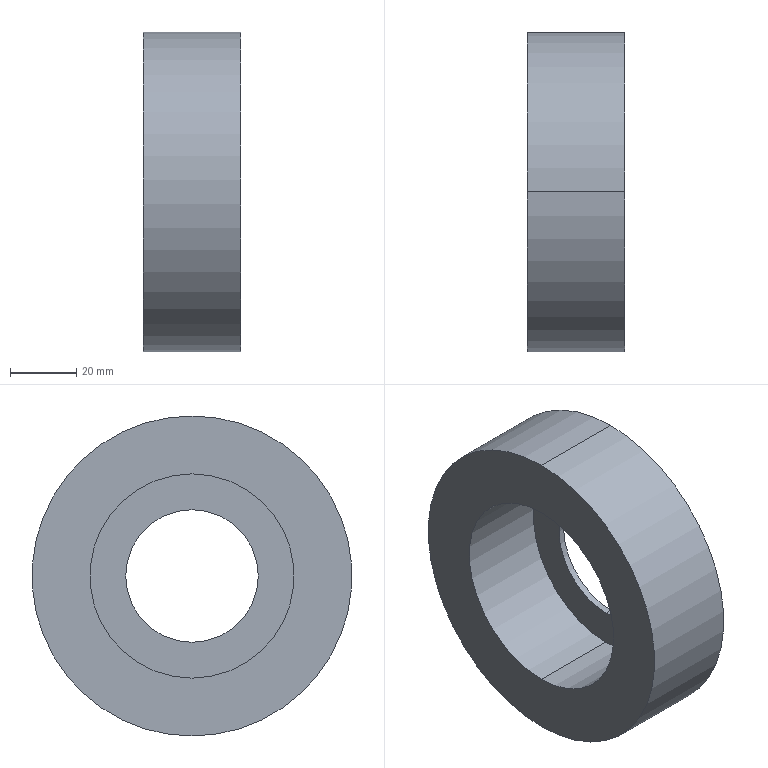Part | STEP file | Market stator | 1 solid | 9 faces | box 29.5 x 96.5 x 96.5 mm | volume 131288 mm3 | cylinder 6 | plane 3 | commonest cylinder face diameters 40 x2 61.6 x2 96.5 x2
STEP:
#1=CARTESIAN_POINT('',(0.,0.,0.));
#2=DIRECTION('',(0.,0.,1.));
#3=DIRECTION('',(1.,0.,0.));
#4=AXIS2_PLACEMENT_3D('',#1,#2,#3);
#5=CARTESIAN_POINT('',(-2.,0.,-20.));
#6=VERTEX_POINT('',#5);
#7=CARTESIAN_POINT('',(0.,0.,-20.));
#8=VERTEX_POINT('',#7);
#9=CARTESIAN_POINT('',(0.,0.,-20.));
#10=DIRECTION('',(1.,0.,0.));
#11=VECTOR('',#10,1.);
#12=LINE('',#9,#11);
#13=CARTESIAN_POINT('',(0.,0.,0.));
#14=DIRECTION('',(1.,0.,0.));
#15=DIRECTION('',(0.,0.,-1.));
#16=AXIS2_PLACEMENT_3D('',#13,#14,#15);
#17=CYLINDRICAL_SURFACE('',#16,20.);
#18=CARTESIAN_POINT('',(6.283,0.));
#19=DIRECTION('',(0.,1.));
#20=VECTOR('',#19,1.);
#21=LINE('',#18,#20);
#22=(GEOMETRIC_REPRESENTATION_CONTEXT(2)PARAMETRIC_REPRESENTATION_CONTEXT()REPRESENTATION_CONTEXT('',''));
#23=DEFINITIONAL_REPRESENTATION('',(#21),#22);
#24=PCURVE('',#17,#23);
#25=CARTESIAN_POINT('',(0.,0.,0.));
#26=DIRECTION('',(1.,0.,0.));
#27=DIRECTION('',(0.,0.,-1.));
#28=AXIS2_PLACEMENT_3D('',#25,#26,#27);
#29=CYLINDRICAL_SURFACE('',#28,20.);
#30=CARTESIAN_POINT('',(0.,0.));
#31=DIRECTION('',(0.,1.));
#32=VECTOR('',#31,1.);
#33=LINE('',#30,#32);
#34=(GEOMETRIC_REPRESENTATION_CONTEXT(2)PARAMETRIC_REPRESENTATION_CONTEXT()REPRESENTATION_CONTEXT('',''));
#35=DEFINITIONAL_REPRESENTATION('',(#33),#34);
#36=PCURVE('',#29,#35);
#37=SURFACE_CURVE('',#12,(#24,#36),.PCURVE_S1.);
#38=EDGE_CURVE('',#6,#8,#37,.T.);
#39=ORIENTED_EDGE('',*,*,#38,.T.);
#40=CARTESIAN_POINT('',(0.,0.,20.));
#41=VERTEX_POINT('',#40);
#42=CARTESIAN_POINT('',(0.,0.,0.));
#43=DIRECTION('',(-1.,0.,0.));
#44=DIRECTION('',(0.,0.,-1.));
#45=AXIS2_PLACEMENT_3D('',#42,#43,#44);
#46=CIRCLE('',#45,20.);
#47=CARTESIAN_POINT('',(6.283,0.));
#48=DIRECTION('',(-1.,0.));
#49=VECTOR('',#48,1.);
#50=LINE('',#47,#49);
#51=(GEOMETRIC_REPRESENTATION_CONTEXT(2)PARAMETRIC_REPRESENTATION_CONTEXT()REPRESENTATION_CONTEXT('',''));
#52=DEFINITIONAL_REPRESENTATION('',(#50),#51);
#53=PCURVE('',#17,#52);
#54=CARTESIAN_POINT('',(0.,20.,0.));
#55=DIRECTION('',(1.,0.,0.));
#56=DIRECTION('',(0.,0.,-1.));
#57=AXIS2_PLACEMENT_3D('',#54,#55,#56);
#58=PLANE('',#57);
#59=CARTESIAN_POINT('',(20.,-20.));
#60=CARTESIAN_POINT('',(20.,-54.641));
#61=CARTESIAN_POINT('',(-10.,-37.321));
#62=CARTESIAN_POINT('',(-40.,-20.));
#63=CARTESIAN_POINT('',(-10.,-2.679));
#64=CARTESIAN_POINT('',(20.,14.641));
#65=CARTESIAN_POINT('',(20.,-20.));
#66=(BOUNDED_CURVE()B_SPLINE_CURVE(2,(#59,#60,#61,#62,#63,#64,#65),.UNSPECIFIED.,.T.,.F.)B_SPLINE_CURVE_WITH_KNOTS((1,2,2,2,2,1),(-2.094,0.,2.094,4.189,6.283,8.378),.UNSPECIFIED.)CURVE()GEOMETRIC_REPRESENTATION_ITEM()RATIONAL_B_SPLINE_CURVE((1.,0.5,1.,0.5,1.,0.5,1.))REPRESENTATION_ITEM(''));
#67=(GEOMETRIC_REPRESENTATION_CONTEXT(2)PARAMETRIC_REPRESENTATION_CONTEXT()REPRESENTATION_CONTEXT('',''));
#68=DEFINITIONAL_REPRESENTATION('',(#66),#67);
#69=PCURVE('',#58,#68);
#70=SURFACE_CURVE('',#46,(#53,#69),.PCURVE_S1.);
#71=EDGE_CURVE('',#8,#41,#70,.T.);
#72=ORIENTED_EDGE('',*,*,#71,.T.);
#73=CARTESIAN_POINT('',(-2.,0.,20.));
#74=VERTEX_POINT('',#73);
#75=CARTESIAN_POINT('',(0.,0.,20.));
#76=DIRECTION('',(1.,0.,0.));
#77=VECTOR('',#76,1.);
#78=LINE('',#75,#77);
#79=CARTESIAN_POINT('',(3.142,0.));
#80=DIRECTION('',(0.,1.));
#81=VECTOR('',#80,1.);
#82=LINE('',#79,#81);
#83=(GEOMETRIC_REPRESENTATION_CONTEXT(2)PARAMETRIC_REPRESENTATION_CONTEXT()REPRESENTATION_CONTEXT('',''));
#84=DEFINITIONAL_REPRESENTATION('',(#82),#83);
#85=PCURVE('',#17,#84);
#86=CARTESIAN_POINT('',(3.142,0.));
#87=DIRECTION('',(0.,1.));
#88=VECTOR('',#87,1.);
#89=LINE('',#86,#88);
#90=(GEOMETRIC_REPRESENTATION_CONTEXT(2)PARAMETRIC_REPRESENTATION_CONTEXT()REPRESENTATION_CONTEXT('',''));
#91=DEFINITIONAL_REPRESENTATION('',(#89),#90);
#92=PCURVE('',#29,#91);
#93=SURFACE_CURVE('',#78,(#85,#92),.PCURVE_S1.);
#94=EDGE_CURVE('',#74,#41,#93,.T.);
#95=ORIENTED_EDGE('',*,*,#94,.F.);
#96=CARTESIAN_POINT('',(-2.,0.,0.));
#97=DIRECTION('',(1.,0.,0.));
#98=DIRECTION('',(0.,0.,-1.));
#99=AXIS2_PLACEMENT_3D('',#96,#97,#98);
#100=CIRCLE('',#99,20.);
#101=CARTESIAN_POINT('',(0.,-2.));
#102=DIRECTION('',(1.,0.));
#103=VECTOR('',#102,1.);
#104=LINE('',#101,#103);
#105=(GEOMETRIC_REPRESENTATION_CONTEXT(2)PARAMETRIC_REPRESENTATION_CONTEXT()REPRESENTATION_CONTEXT('',''));
#106=DEFINITIONAL_REPRESENTATION('',(#104),#105);
#107=PCURVE('',#17,#106);
#108=CARTESIAN_POINT('',(-2.,30.8,0.));
#109=DIRECTION('',(-1.,0.,0.));
#110=DIRECTION('',(0.,0.,1.));
#111=AXIS2_PLACEMENT_3D('',#108,#109,#110);
#112=PLANE('',#111);
#113=CARTESIAN_POINT('',(-20.,-30.8));
#114=CARTESIAN_POINT('',(-20.,3.841));
#115=CARTESIAN_POINT('',(10.,-13.479));
#116=CARTESIAN_POINT('',(40.,-30.8));
#117=CARTESIAN_POINT('',(10.,-48.121));
#118=CARTESIAN_POINT('',(-20.,-65.441));
#119=CARTESIAN_POINT('',(-20.,-30.8));
#120=(BOUNDED_CURVE()B_SPLINE_CURVE(2,(#113,#114,#115,#116,#117,#118,#119),.UNSPECIFIED.,.T.,.F.)B_SPLINE_CURVE_WITH_KNOTS((1,2,2,2,2,1),(-2.094,0.,2.094,4.189,6.283,8.378),.UNSPECIFIED.)CURVE()GEOMETRIC_REPRESENTATION_ITEM()RATIONAL_B_SPLINE_CURVE((1.,0.5,1.,0.5,1.,0.5,1.))REPRESENTATION_ITEM(''));
#121=(GEOMETRIC_REPRESENTATION_CONTEXT(2)PARAMETRIC_REPRESENTATION_CONTEXT()REPRESENTATION_CONTEXT('',''));
#122=DEFINITIONAL_REPRESENTATION('',(#120),#121);
#123=PCURVE('',#112,#122);
#124=SURFACE_CURVE('',#100,(#107,#123),.PCURVE_S1.);
#125=EDGE_CURVE('',#74,#6,#124,.T.);
#126=ORIENTED_EDGE('',*,*,#125,.T.);
#127=EDGE_LOOP('',(#39,#72,#95,#126));
#128=FACE_BOUND('',#127,.F.);
#129=ADVANCED_FACE('',(#128),#17,.F.);
#130=CARTESIAN_POINT('',(-29.5,0.,-48.25));
#131=VERTEX_POINT('',#130);
#132=CARTESIAN_POINT('',(-29.5,0.,48.25));
#133=VERTEX_POINT('',#132);
#134=CARTESIAN_POINT('',(-29.5,0.,0.));
#135=DIRECTION('',(1.,0.,0.));
#136=DIRECTION('',(0.,0.,-1.));
#137=AXIS2_PLACEMENT_3D('',#134,#135,#136);
#138=CIRCLE('',#137,48.25);
#139=CARTESIAN_POINT('',(0.,0.,0.));
#140=DIRECTION('',(1.,0.,0.));
#141=DIRECTION('',(0.,0.,-1.));
#142=AXIS2_PLACEMENT_3D('',#139,#140,#141);
#143=CYLINDRICAL_SURFACE('',#142,48.25);
#144=CARTESIAN_POINT('',(0.,-29.5));
#145=DIRECTION('',(1.,0.));
#146=VECTOR('',#145,1.);
#147=LINE('',#144,#146);
#148=(GEOMETRIC_REPRESENTATION_CONTEXT(2)PARAMETRIC_REPRESENTATION_CONTEXT()REPRESENTATION_CONTEXT('',''));
#149=DEFINITIONAL_REPRESENTATION('',(#147),#148);
#150=PCURVE('',#143,#149);
#151=CARTESIAN_POINT('',(-29.5,48.25,0.));
#152=DIRECTION('',(-1.,0.,0.));
#153=DIRECTION('',(0.,0.,1.));
#154=AXIS2_PLACEMENT_3D('',#151,#152,#153);
#155=PLANE('',#154);
#156=CARTESIAN_POINT('',(-48.25,-48.25));
#157=CARTESIAN_POINT('',(-48.25,35.321));
#158=CARTESIAN_POINT('',(24.125,-6.464));
#159=CARTESIAN_POINT('',(96.5,-48.25));
#160=CARTESIAN_POINT('',(24.125,-90.036));
#161=CARTESIAN_POINT('',(-48.25,-131.821));
#162=CARTESIAN_POINT('',(-48.25,-48.25));
#163=(BOUNDED_CURVE()B_SPLINE_CURVE(2,(#156,#157,#158,#159,#160,#161,#162),.UNSPECIFIED.,.T.,.F.)B_SPLINE_CURVE_WITH_KNOTS((1,2,2,2,2,1),(-2.094,0.,2.094,4.189,6.283,8.378),.UNSPECIFIED.)CURVE()GEOMETRIC_REPRESENTATION_ITEM()RATIONAL_B_SPLINE_CURVE((1.,0.5,1.,0.5,1.,0.5,1.))REPRESENTATION_ITEM(''));
#164=(GEOMETRIC_REPRESENTATION_CONTEXT(2)PARAMETRIC_REPRESENTATION_CONTEXT()REPRESENTATION_CONTEXT('',''));
#165=DEFINITIONAL_REPRESENTATION('',(#163),#164);
#166=PCURVE('',#155,#165);
#167=SURFACE_CURVE('',#138,(#150,#166),.PCURVE_S1.);
#168=EDGE_CURVE('',#131,#133,#167,.T.);
#169=ORIENTED_EDGE('',*,*,#168,.T.);
#170=CARTESIAN_POINT('',(0.,0.,48.25));
#171=VERTEX_POINT('',#170);
#172=CARTESIAN_POINT('',(0.,0.,48.25));
#173=DIRECTION('',(1.,0.,0.));
#174=VECTOR('',#173,1.);
#175=LINE('',#172,#174);
#176=CARTESIAN_POINT('',(3.142,0.));
#177=DIRECTION('',(0.,1.));
#178=VECTOR('',#177,1.);
#179=LINE('',#176,#178);
#180=(GEOMETRIC_REPRESENTATION_CONTEXT(2)PARAMETRIC_REPRESENTATION_CONTEXT()REPRESENTATION_CONTEXT('',''));
#181=DEFINITIONAL_REPRESENTATION('',(#179),#180);
#182=PCURVE('',#143,#181);
#183=CARTESIAN_POINT('',(0.,0.,0.));
#184=DIRECTION('',(1.,0.,0.));
#185=DIRECTION('',(0.,0.,-1.));
#186=AXIS2_PLACEMENT_3D('',#183,#184,#185);
#187=CYLINDRICAL_SURFACE('',#186,48.25);
#188=CARTESIAN_POINT('',(3.142,0.));
#189=DIRECTION('',(0.,1.));
#190=VECTOR('',#189,1.);
#191=LINE('',#188,#190);
#192=(GEOMETRIC_REPRESENTATION_CONTEXT(2)PARAMETRIC_REPRESENTATION_CONTEXT()REPRESENTATION_CONTEXT('',''));
#193=DEFINITIONAL_REPRESENTATION('',(#191),#192);
#194=PCURVE('',#187,#193);
#195=SURFACE_CURVE('',#175,(#182,#194),.PCURVE_S1.);
#196=EDGE_CURVE('',#133,#171,#195,.T.);
#197=ORIENTED_EDGE('',*,*,#196,.T.);
#198=CARTESIAN_POINT('',(0.,0.,-48.25));
#199=VERTEX_POINT('',#198);
#200=CARTESIAN_POINT('',(0.,0.,0.));
#201=DIRECTION('',(1.,0.,0.));
#202=DIRECTION('',(0.,0.,-1.));
#203=AXIS2_PLACEMENT_3D('',#200,#201,#202);
#204=CIRCLE('',#203,48.25);
#205=CARTESIAN_POINT('',(0.,0.));
#206=DIRECTION('',(1.,0.));
#207=VECTOR('',#206,1.);
#208=LINE('',#205,#207);
#209=(GEOMETRIC_REPRESENTATION_CONTEXT(2)PARAMETRIC_REPRESENTATION_CONTEXT()REPRESENTATION_CONTEXT('',''));
#210=DEFINITIONAL_REPRESENTATION('',(#208),#209);
#211=PCURVE('',#143,#210);
#212=CARTESIAN_POINT('',(0.,-20.));
#213=DIRECTION('',(1.,0.));
#214=AXIS2_PLACEMENT_2D('',#212,#213);
#215=CIRCLE('',#214,48.25);
#216=(GEOMETRIC_REPRESENTATION_CONTEXT(2)PARAMETRIC_REPRESENTATION_CONTEXT()REPRESENTATION_CONTEXT('',''));
#217=DEFINITIONAL_REPRESENTATION('',(#215),#216);
#218=PCURVE('',#58,#217);
#219=SURFACE_CURVE('',#204,(#211,#218),.PCURVE_S1.);
#220=EDGE_CURVE('',#199,#171,#219,.T.);
#221=ORIENTED_EDGE('',*,*,#220,.F.);
#222=CARTESIAN_POINT('',(0.,0.,-48.25));
#223=DIRECTION('',(1.,0.,0.));
#224=VECTOR('',#223,1.);
#225=LINE('',#222,#224);
#226=CARTESIAN_POINT('',(0.,0.));
#227=DIRECTION('',(0.,1.));
#228=VECTOR('',#227,1.);
#229=LINE('',#226,#228);
#230=(GEOMETRIC_REPRESENTATION_CONTEXT(2)PARAMETRIC_REPRESENTATION_CONTEXT()REPRESENTATION_CONTEXT('',''));
#231=DEFINITIONAL_REPRESENTATION('',(#229),#230);
#232=PCURVE('',#143,#231);
#233=CARTESIAN_POINT('',(6.283,0.));
#234=DIRECTION('',(0.,1.));
#235=VECTOR('',#234,1.);
#236=LINE('',#233,#235);
#237=(GEOMETRIC_REPRESENTATION_CONTEXT(2)PARAMETRIC_REPRESENTATION_CONTEXT()REPRESENTATION_CONTEXT('',''));
#238=DEFINITIONAL_REPRESENTATION('',(#236),#237);
#239=PCURVE('',#187,#238);
#240=SURFACE_CURVE('',#225,(#232,#239),.PCURVE_S1.);
#241=EDGE_CURVE('',#131,#199,#240,.T.);
#242=ORIENTED_EDGE('',*,*,#241,.F.);
#243=EDGE_LOOP('',(#169,#197,#221,#242));
#244=FACE_BOUND('',#243,.T.);
#245=ADVANCED_FACE('',(#244),#143,.T.);
#246=CARTESIAN_POINT('',(-29.5,0.,-30.8));
#247=VERTEX_POINT('',#246);
#248=CARTESIAN_POINT('',(-2.,0.,-30.8));
#249=VERTEX_POINT('',#248);
#250=CARTESIAN_POINT('',(0.,0.,-30.8));
#251=DIRECTION('',(1.,0.,0.));
#252=VECTOR('',#251,1.);
#253=LINE('',#250,#252);
#254=CARTESIAN_POINT('',(0.,0.,0.));
#255=DIRECTION('',(1.,0.,0.));
#256=DIRECTION('',(0.,0.,-1.));
#257=AXIS2_PLACEMENT_3D('',#254,#255,#256);
#258=CYLINDRICAL_SURFACE('',#257,30.8);
#259=CARTESIAN_POINT('',(6.283,0.));
#260=DIRECTION('',(0.,1.));
#261=VECTOR('',#260,1.);
#262=LINE('',#259,#261);
#263=(GEOMETRIC_REPRESENTATION_CONTEXT(2)PARAMETRIC_REPRESENTATION_CONTEXT()REPRESENTATION_CONTEXT('',''));
#264=DEFINITIONAL_REPRESENTATION('',(#262),#263);
#265=PCURVE('',#258,#264);
#266=CARTESIAN_POINT('',(0.,0.,0.));
#267=DIRECTION('',(1.,0.,0.));
#268=DIRECTION('',(0.,0.,-1.));
#269=AXIS2_PLACEMENT_3D('',#266,#267,#268);
#270=CYLINDRICAL_SURFACE('',#269,30.8);
#271=CARTESIAN_POINT('',(0.,0.));
#272=DIRECTION('',(0.,1.));
#273=VECTOR('',#272,1.);
#274=LINE('',#271,#273);
#275=(GEOMETRIC_REPRESENTATION_CONTEXT(2)PARAMETRIC_REPRESENTATION_CONTEXT()REPRESENTATION_CONTEXT('',''));
#276=DEFINITIONAL_REPRESENTATION('',(#274),#275);
#277=PCURVE('',#270,#276);
#278=SURFACE_CURVE('',#253,(#265,#277),.PCURVE_S1.);
#279=EDGE_CURVE('',#247,#249,#278,.T.);
#280=ORIENTED_EDGE('',*,*,#279,.T.);
#281=CARTESIAN_POINT('',(-2.,0.,30.8));
#282=VERTEX_POINT('',#281);
#283=CARTESIAN_POINT('',(-2.,0.,0.));
#284=DIRECTION('',(-1.,0.,0.));
#285=DIRECTION('',(0.,0.,-1.));
#286=AXIS2_PLACEMENT_3D('',#283,#284,#285);
#287=CIRCLE('',#286,30.8);
#288=CARTESIAN_POINT('',(6.283,-2.));
#289=DIRECTION('',(-1.,0.));
#290=VECTOR('',#289,1.);
#291=LINE('',#288,#290);
#292=(GEOMETRIC_REPRESENTATION_CONTEXT(2)PARAMETRIC_REPRESENTATION_CONTEXT()REPRESENTATION_CONTEXT('',''));
#293=DEFINITIONAL_REPRESENTATION('',(#291),#292);
#294=PCURVE('',#258,#293);
#295=CARTESIAN_POINT('',(0.,-30.8));
#296=DIRECTION('',(-1.,0.));
#297=AXIS2_PLACEMENT_2D('',#295,#296);
#298=CIRCLE('',#297,30.8);
#299=(GEOMETRIC_REPRESENTATION_CONTEXT(2)PARAMETRIC_REPRESENTATION_CONTEXT()REPRESENTATION_CONTEXT('',''));
#300=DEFINITIONAL_REPRESENTATION('',(#298),#299);
#301=PCURVE('',#112,#300);
#302=SURFACE_CURVE('',#287,(#294,#301),.PCURVE_S1.);
#303=EDGE_CURVE('',#249,#282,#302,.T.);
#304=ORIENTED_EDGE('',*,*,#303,.T.);
#305=CARTESIAN_POINT('',(-29.5,0.,30.8));
#306=VERTEX_POINT('',#305);
#307=CARTESIAN_POINT('',(0.,0.,30.8));
#308=DIRECTION('',(1.,0.,0.));
#309=VECTOR('',#308,1.);
#310=LINE('',#307,#309);
#311=CARTESIAN_POINT('',(3.142,0.));
#312=DIRECTION('',(0.,1.));
#313=VECTOR('',#312,1.);
#314=LINE('',#311,#313);
#315=(GEOMETRIC_REPRESENTATION_CONTEXT(2)PARAMETRIC_REPRESENTATION_CONTEXT()REPRESENTATION_CONTEXT('',''));
#316=DEFINITIONAL_REPRESENTATION('',(#314),#315);
#317=PCURVE('',#258,#316);
#318=CARTESIAN_POINT('',(3.142,0.));
#319=DIRECTION('',(0.,1.));
#320=VECTOR('',#319,1.);
#321=LINE('',#318,#320);
#322=(GEOMETRIC_REPRESENTATION_CONTEXT(2)PARAMETRIC_REPRESENTATION_CONTEXT()REPRESENTATION_CONTEXT('',''));
#323=DEFINITIONAL_REPRESENTATION('',(#321),#322);
#324=PCURVE('',#270,#323);
#325=SURFACE_CURVE('',#310,(#317,#324),.PCURVE_S1.);
#326=EDGE_CURVE('',#306,#282,#325,.T.);
#327=ORIENTED_EDGE('',*,*,#326,.F.);
#328=CARTESIAN_POINT('',(-29.5,0.,0.));
#329=DIRECTION('',(1.,0.,0.));
#330=DIRECTION('',(0.,0.,-1.));
#331=AXIS2_PLACEMENT_3D('',#328,#329,#330);
#332=CIRCLE('',#331,30.8);
#333=CARTESIAN_POINT('',(0.,-29.5));
#334=DIRECTION('',(1.,0.));
#335=VECTOR('',#334,1.);
#336=LINE('',#333,#335);
#337=(GEOMETRIC_REPRESENTATION_CONTEXT(2)PARAMETRIC_REPRESENTATION_CONTEXT()REPRESENTATION_CONTEXT('',''));
#338=DEFINITIONAL_REPRESENTATION('',(#336),#337);
#339=PCURVE('',#258,#338);
#340=CARTESIAN_POINT('',(-30.8,-48.25));
#341=CARTESIAN_POINT('',(-30.8,5.097));
#342=CARTESIAN_POINT('',(15.4,-21.576));
#343=CARTESIAN_POINT('',(61.6,-48.25));
#344=CARTESIAN_POINT('',(15.4,-74.924));
#345=CARTESIAN_POINT('',(-30.8,-101.597));
#346=CARTESIAN_POINT('',(-30.8,-48.25));
#347=(BOUNDED_CURVE()B_SPLINE_CURVE(2,(#340,#341,#342,#343,#344,#345,#346),.UNSPECIFIED.,.T.,.F.)B_SPLINE_CURVE_WITH_KNOTS((1,2,2,2,2,1),(-2.094,0.,2.094,4.189,6.283,8.378),.UNSPECIFIED.)CURVE()GEOMETRIC_REPRESENTATION_ITEM()RATIONAL_B_SPLINE_CURVE((1.,0.5,1.,0.5,1.,0.5,1.))REPRESENTATION_ITEM(''));
#348=(GEOMETRIC_REPRESENTATION_CONTEXT(2)PARAMETRIC_REPRESENTATION_CONTEXT()REPRESENTATION_CONTEXT('',''));
#349=DEFINITIONAL_REPRESENTATION('',(#347),#348);
#350=PCURVE('',#155,#349);
#351=SURFACE_CURVE('',#332,(#339,#350),.PCURVE_S1.);
#352=EDGE_CURVE('',#306,#247,#351,.T.);
#353=ORIENTED_EDGE('',*,*,#352,.T.);
#354=EDGE_LOOP('',(#280,#304,#327,#353));
#355=FACE_BOUND('',#354,.F.);
#356=ADVANCED_FACE('',(#355),#258,.F.);
#357=ORIENTED_EDGE('',*,*,#71,.T.);
#358=CARTESIAN_POINT('',(0.,0.,0.));
#359=DIRECTION('',(-1.,0.,0.));
#360=DIRECTION('',(0.,0.,-1.));
#361=AXIS2_PLACEMENT_3D('',#358,#359,#360);
#362=CIRCLE('',#361,20.);
#363=CARTESIAN_POINT('',(20.,-20.));
#364=CARTESIAN_POINT('',(20.,-54.641));
#365=CARTESIAN_POINT('',(-10.,-37.321));
#366=CARTESIAN_POINT('',(-40.,-20.));
#367=CARTESIAN_POINT('',(-10.,-2.679));
#368=CARTESIAN_POINT('',(20.,14.641));
#369=CARTESIAN_POINT('',(20.,-20.));
#370=(BOUNDED_CURVE()B_SPLINE_CURVE(2,(#363,#364,#365,#366,#367,#368,#369),.UNSPECIFIED.,.T.,.F.)B_SPLINE_CURVE_WITH_KNOTS((1,2,2,2,2,1),(-2.094,0.,2.094,4.189,6.283,8.378),.UNSPECIFIED.)CURVE()GEOMETRIC_REPRESENTATION_ITEM()RATIONAL_B_SPLINE_CURVE((1.,0.5,1.,0.5,1.,0.5,1.))REPRESENTATION_ITEM(''));
#371=(GEOMETRIC_REPRESENTATION_CONTEXT(2)PARAMETRIC_REPRESENTATION_CONTEXT()REPRESENTATION_CONTEXT('',''));
#372=DEFINITIONAL_REPRESENTATION('',(#370),#371);
#373=PCURVE('',#58,#372);
#374=CARTESIAN_POINT('',(6.283,0.));
#375=DIRECTION('',(-1.,0.));
#376=VECTOR('',#375,1.);
#377=LINE('',#374,#376);
#378=(GEOMETRIC_REPRESENTATION_CONTEXT(2)PARAMETRIC_REPRESENTATION_CONTEXT()REPRESENTATION_CONTEXT('',''));
#379=DEFINITIONAL_REPRESENTATION('',(#377),#378);
#380=PCURVE('',#29,#379);
#381=SURFACE_CURVE('',#362,(#373,#380),.PCURVE_S1.);
#382=EDGE_CURVE('',#41,#8,#381,.T.);
#383=ORIENTED_EDGE('',*,*,#382,.T.);
#384=EDGE_LOOP('',(#357,#383));
#385=FACE_BOUND('',#384,.T.);
#386=ORIENTED_EDGE('',*,*,#220,.T.);
#387=CARTESIAN_POINT('',(0.,0.,0.));
#388=DIRECTION('',(1.,0.,0.));
#389=DIRECTION('',(0.,0.,-1.));
#390=AXIS2_PLACEMENT_3D('',#387,#388,#389);
#391=CIRCLE('',#390,48.25);
#392=CARTESIAN_POINT('',(0.,-20.));
#393=DIRECTION('',(1.,0.));
#394=AXIS2_PLACEMENT_2D('',#392,#393);
#395=CIRCLE('',#394,48.25);
#396=(GEOMETRIC_REPRESENTATION_CONTEXT(2)PARAMETRIC_REPRESENTATION_CONTEXT()REPRESENTATION_CONTEXT('',''));
#397=DEFINITIONAL_REPRESENTATION('',(#395),#396);
#398=PCURVE('',#58,#397);
#399=CARTESIAN_POINT('',(0.,0.));
#400=DIRECTION('',(1.,0.));
#401=VECTOR('',#400,1.);
#402=LINE('',#399,#401);
#403=(GEOMETRIC_REPRESENTATION_CONTEXT(2)PARAMETRIC_REPRESENTATION_CONTEXT()REPRESENTATION_CONTEXT('',''));
#404=DEFINITIONAL_REPRESENTATION('',(#402),#403);
#405=PCURVE('',#187,#404);
#406=SURFACE_CURVE('',#391,(#398,#405),.PCURVE_S1.);
#407=EDGE_CURVE('',#171,#199,#406,.T.);
#408=ORIENTED_EDGE('',*,*,#407,.T.);
#409=EDGE_LOOP('',(#386,#408));
#410=FACE_BOUND('',#409,.T.);
#411=ADVANCED_FACE('',(#385,#410),#58,.T.);
#412=ORIENTED_EDGE('',*,*,#382,.T.);
#413=ORIENTED_EDGE('',*,*,#38,.F.);
#414=CARTESIAN_POINT('',(-2.,0.,0.));
#415=DIRECTION('',(1.,0.,0.));
#416=DIRECTION('',(0.,0.,-1.));
#417=AXIS2_PLACEMENT_3D('',#414,#415,#416);
#418=CIRCLE('',#417,20.);
#419=CARTESIAN_POINT('',(0.,-2.));
#420=DIRECTION('',(1.,0.));
#421=VECTOR('',#420,1.);
#422=LINE('',#419,#421);
#423=(GEOMETRIC_REPRESENTATION_CONTEXT(2)PARAMETRIC_REPRESENTATION_CONTEXT()REPRESENTATION_CONTEXT('',''));
#424=DEFINITIONAL_REPRESENTATION('',(#422),#423);
#425=PCURVE('',#29,#424);
#426=CARTESIAN_POINT('',(-20.,-30.8));
#427=CARTESIAN_POINT('',(-20.,3.841));
#428=CARTESIAN_POINT('',(10.,-13.479));
#429=CARTESIAN_POINT('',(40.,-30.8));
#430=CARTESIAN_POINT('',(10.,-48.121));
#431=CARTESIAN_POINT('',(-20.,-65.441));
#432=CARTESIAN_POINT('',(-20.,-30.8));
#433=(BOUNDED_CURVE()B_SPLINE_CURVE(2,(#426,#427,#428,#429,#430,#431,#432),.UNSPECIFIED.,.T.,.F.)B_SPLINE_CURVE_WITH_KNOTS((1,2,2,2,2,1),(-2.094,0.,2.094,4.189,6.283,8.378),.UNSPECIFIED.)CURVE()GEOMETRIC_REPRESENTATION_ITEM()RATIONAL_B_SPLINE_CURVE((1.,0.5,1.,0.5,1.,0.5,1.))REPRESENTATION_ITEM(''));
#434=(GEOMETRIC_REPRESENTATION_CONTEXT(2)PARAMETRIC_REPRESENTATION_CONTEXT()REPRESENTATION_CONTEXT('',''));
#435=DEFINITIONAL_REPRESENTATION('',(#433),#434);
#436=PCURVE('',#112,#435);
#437=SURFACE_CURVE('',#418,(#425,#436),.PCURVE_S1.);
#438=EDGE_CURVE('',#6,#74,#437,.T.);
#439=ORIENTED_EDGE('',*,*,#438,.T.);
#440=ORIENTED_EDGE('',*,*,#94,.T.);
#441=EDGE_LOOP('',(#412,#413,#439,#440));
#442=FACE_BOUND('',#441,.F.);
#443=ADVANCED_FACE('',(#442),#29,.F.);
#444=ORIENTED_EDGE('',*,*,#196,.F.);
#445=CARTESIAN_POINT('',(-29.5,0.,0.));
#446=DIRECTION('',(1.,0.,0.));
#447=DIRECTION('',(0.,0.,-1.));
#448=AXIS2_PLACEMENT_3D('',#445,#446,#447);
#449=CIRCLE('',#448,48.25);
#450=CARTESIAN_POINT('',(0.,-29.5));
#451=DIRECTION('',(1.,0.));
#452=VECTOR('',#451,1.);
#453=LINE('',#450,#452);
#454=(GEOMETRIC_REPRESENTATION_CONTEXT(2)PARAMETRIC_REPRESENTATION_CONTEXT()REPRESENTATION_CONTEXT('',''));
#455=DEFINITIONAL_REPRESENTATION('',(#453),#454);
#456=PCURVE('',#187,#455);
#457=CARTESIAN_POINT('',(-48.25,-48.25));
#458=CARTESIAN_POINT('',(-48.25,35.321));
#459=CARTESIAN_POINT('',(24.125,-6.464));
#460=CARTESIAN_POINT('',(96.5,-48.25));
#461=CARTESIAN_POINT('',(24.125,-90.036));
#462=CARTESIAN_POINT('',(-48.25,-131.821));
#463=CARTESIAN_POINT('',(-48.25,-48.25));
#464=(BOUNDED_CURVE()B_SPLINE_CURVE(2,(#457,#458,#459,#460,#461,#462,#463),.UNSPECIFIED.,.T.,.F.)B_SPLINE_CURVE_WITH_KNOTS((1,2,2,2,2,1),(-2.094,0.,2.094,4.189,6.283,8.378),.UNSPECIFIED.)CURVE()GEOMETRIC_REPRESENTATION_ITEM()RATIONAL_B_SPLINE_CURVE((1.,0.5,1.,0.5,1.,0.5,1.))REPRESENTATION_ITEM(''));
#465=(GEOMETRIC_REPRESENTATION_CONTEXT(2)PARAMETRIC_REPRESENTATION_CONTEXT()REPRESENTATION_CONTEXT('',''));
#466=DEFINITIONAL_REPRESENTATION('',(#464),#465);
#467=PCURVE('',#155,#466);
#468=SURFACE_CURVE('',#449,(#456,#467),.PCURVE_S1.);
#469=EDGE_CURVE('',#133,#131,#468,.T.);
#470=ORIENTED_EDGE('',*,*,#469,.T.);
#471=ORIENTED_EDGE('',*,*,#241,.T.);
#472=ORIENTED_EDGE('',*,*,#407,.F.);
#473=EDGE_LOOP('',(#444,#470,#471,#472));
#474=FACE_BOUND('',#473,.T.);
#475=ADVANCED_FACE('',(#474),#187,.T.);
#476=ORIENTED_EDGE('',*,*,#303,.T.);
#477=CARTESIAN_POINT('',(-2.,0.,0.));
#478=DIRECTION('',(-1.,0.,0.));
#479=DIRECTION('',(0.,0.,-1.));
#480=AXIS2_PLACEMENT_3D('',#477,#478,#479);
#481=CIRCLE('',#480,30.8);
#482=CARTESIAN_POINT('',(0.,-30.8));
#483=DIRECTION('',(-1.,0.));
#484=AXIS2_PLACEMENT_2D('',#482,#483);
#485=CIRCLE('',#484,30.8);
#486=(GEOMETRIC_REPRESENTATION_CONTEXT(2)PARAMETRIC_REPRESENTATION_CONTEXT()REPRESENTATION_CONTEXT('',''));
#487=DEFINITIONAL_REPRESENTATION('',(#485),#486);
#488=PCURVE('',#112,#487);
#489=CARTESIAN_POINT('',(6.283,-2.));
#490=DIRECTION('',(-1.,0.));
#491=VECTOR('',#490,1.);
#492=LINE('',#489,#491);
#493=(GEOMETRIC_REPRESENTATION_CONTEXT(2)PARAMETRIC_REPRESENTATION_CONTEXT()REPRESENTATION_CONTEXT('',''));
#494=DEFINITIONAL_REPRESENTATION('',(#492),#493);
#495=PCURVE('',#270,#494);
#496=SURFACE_CURVE('',#481,(#488,#495),.PCURVE_S1.);
#497=EDGE_CURVE('',#282,#249,#496,.T.);
#498=ORIENTED_EDGE('',*,*,#497,.T.);
#499=EDGE_LOOP('',(#476,#498));
#500=FACE_BOUND('',#499,.T.);
#501=ORIENTED_EDGE('',*,*,#438,.T.);
#502=ORIENTED_EDGE('',*,*,#125,.T.);
#503=EDGE_LOOP('',(#501,#502));
#504=FACE_BOUND('',#503,.T.);
#505=ADVANCED_FACE('',(#500,#504),#112,.T.);
#506=ORIENTED_EDGE('',*,*,#168,.F.);
#507=ORIENTED_EDGE('',*,*,#469,.F.);
#508=EDGE_LOOP('',(#506,#507));
#509=FACE_BOUND('',#508,.T.);
#510=CARTESIAN_POINT('',(-29.5,0.,0.));
#511=DIRECTION('',(1.,0.,0.));
#512=DIRECTION('',(0.,0.,-1.));
#513=AXIS2_PLACEMENT_3D('',#510,#511,#512);
#514=CIRCLE('',#513,30.8);
#515=CARTESIAN_POINT('',(-30.8,-48.25));
#516=CARTESIAN_POINT('',(-30.8,5.097));
#517=CARTESIAN_POINT('',(15.4,-21.576));
#518=CARTESIAN_POINT('',(61.6,-48.25));
#519=CARTESIAN_POINT('',(15.4,-74.924));
#520=CARTESIAN_POINT('',(-30.8,-101.597));
#521=CARTESIAN_POINT('',(-30.8,-48.25));
#522=(BOUNDED_CURVE()B_SPLINE_CURVE(2,(#515,#516,#517,#518,#519,#520,#521),.UNSPECIFIED.,.T.,.F.)B_SPLINE_CURVE_WITH_KNOTS((1,2,2,2,2,1),(-2.094,0.,2.094,4.189,6.283,8.378),.UNSPECIFIED.)CURVE()GEOMETRIC_REPRESENTATION_ITEM()RATIONAL_B_SPLINE_CURVE((1.,0.5,1.,0.5,1.,0.5,1.))REPRESENTATION_ITEM(''));
#523=(GEOMETRIC_REPRESENTATION_CONTEXT(2)PARAMETRIC_REPRESENTATION_CONTEXT()REPRESENTATION_CONTEXT('',''));
#524=DEFINITIONAL_REPRESENTATION('',(#522),#523);
#525=PCURVE('',#155,#524);
#526=CARTESIAN_POINT('',(0.,-29.5));
#527=DIRECTION('',(1.,0.));
#528=VECTOR('',#527,1.);
#529=LINE('',#526,#528);
#530=(GEOMETRIC_REPRESENTATION_CONTEXT(2)PARAMETRIC_REPRESENTATION_CONTEXT()REPRESENTATION_CONTEXT('',''));
#531=DEFINITIONAL_REPRESENTATION('',(#529),#530);
#532=PCURVE('',#270,#531);
#533=SURFACE_CURVE('',#514,(#525,#532),.PCURVE_S1.);
#534=EDGE_CURVE('',#247,#306,#533,.T.);
#535=ORIENTED_EDGE('',*,*,#534,.T.);
#536=ORIENTED_EDGE('',*,*,#352,.T.);
#537=EDGE_LOOP('',(#535,#536));
#538=FACE_BOUND('',#537,.T.);
#539=ADVANCED_FACE('',(#509,#538),#155,.T.);
#540=ORIENTED_EDGE('',*,*,#497,.T.);
#541=ORIENTED_EDGE('',*,*,#279,.F.);
#542=ORIENTED_EDGE('',*,*,#534,.T.);
#543=ORIENTED_EDGE('',*,*,#326,.T.);
#544=EDGE_LOOP('',(#540,#541,#542,#543));
#545=FACE_BOUND('',#544,.F.);
#546=ADVANCED_FACE('',(#545),#270,.F.);
#547=CLOSED_SHELL('',(#129,#245,#356,#411,#443,#475,#505,#539,#546));
#548=MANIFOLD_SOLID_BREP('',#547);
#549=(LENGTH_UNIT()NAMED_UNIT(*)SI_UNIT(.MILLI.,.METRE.));
#550=UNCERTAINTY_MEASURE_WITH_UNIT(LENGTH_MEASURE(0.0000001),#549,'','');
#551=(NAMED_UNIT(*)PLANE_ANGLE_UNIT()SI_UNIT($,.RADIAN.));
#552=(NAMED_UNIT(*)SI_UNIT($,.STERADIAN.)SOLID_ANGLE_UNIT());
#553=(GEOMETRIC_REPRESENTATION_CONTEXT(3)GLOBAL_UNCERTAINTY_ASSIGNED_CONTEXT((#550))GLOBAL_UNIT_ASSIGNED_CONTEXT((#549,#551,#552))REPRESENTATION_CONTEXT('',''));
#554=ADVANCED_BREP_SHAPE_REPRESENTATION('',(#4,#548),#553);